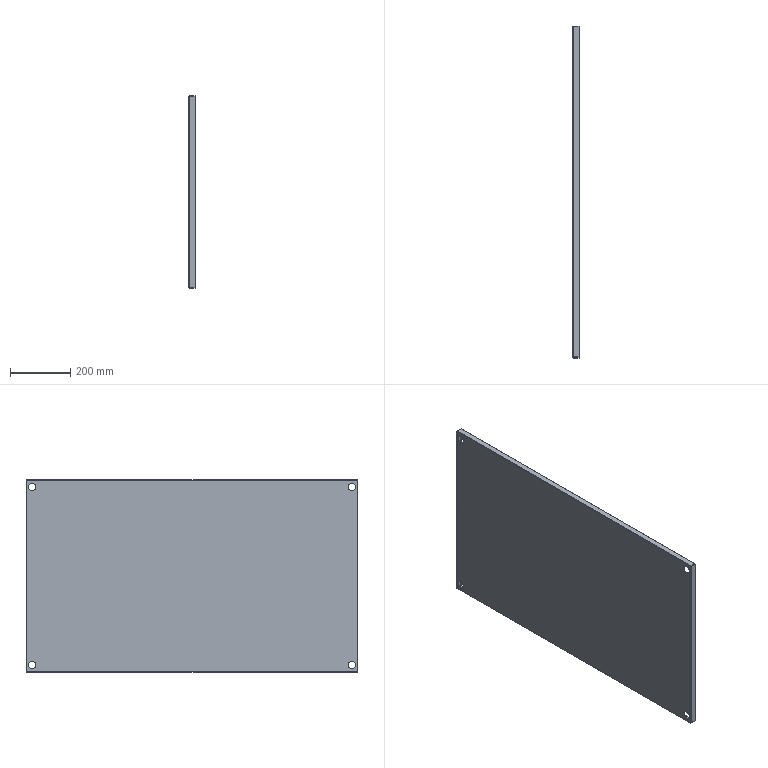Part | SolidWorks | features Cut 1, EdgeFlange 1, FlatPattern 1, SMBaseFlange 1, SheetMetal 1 | 1 solid | 46 faces | box 20 x 1100 x 640 mm | volume 1523319 mm3 | plane 22 | cylinder 16 | spline 8 | commonest cylinder face diameters 25 x8 1.5 x4 5.5 x4